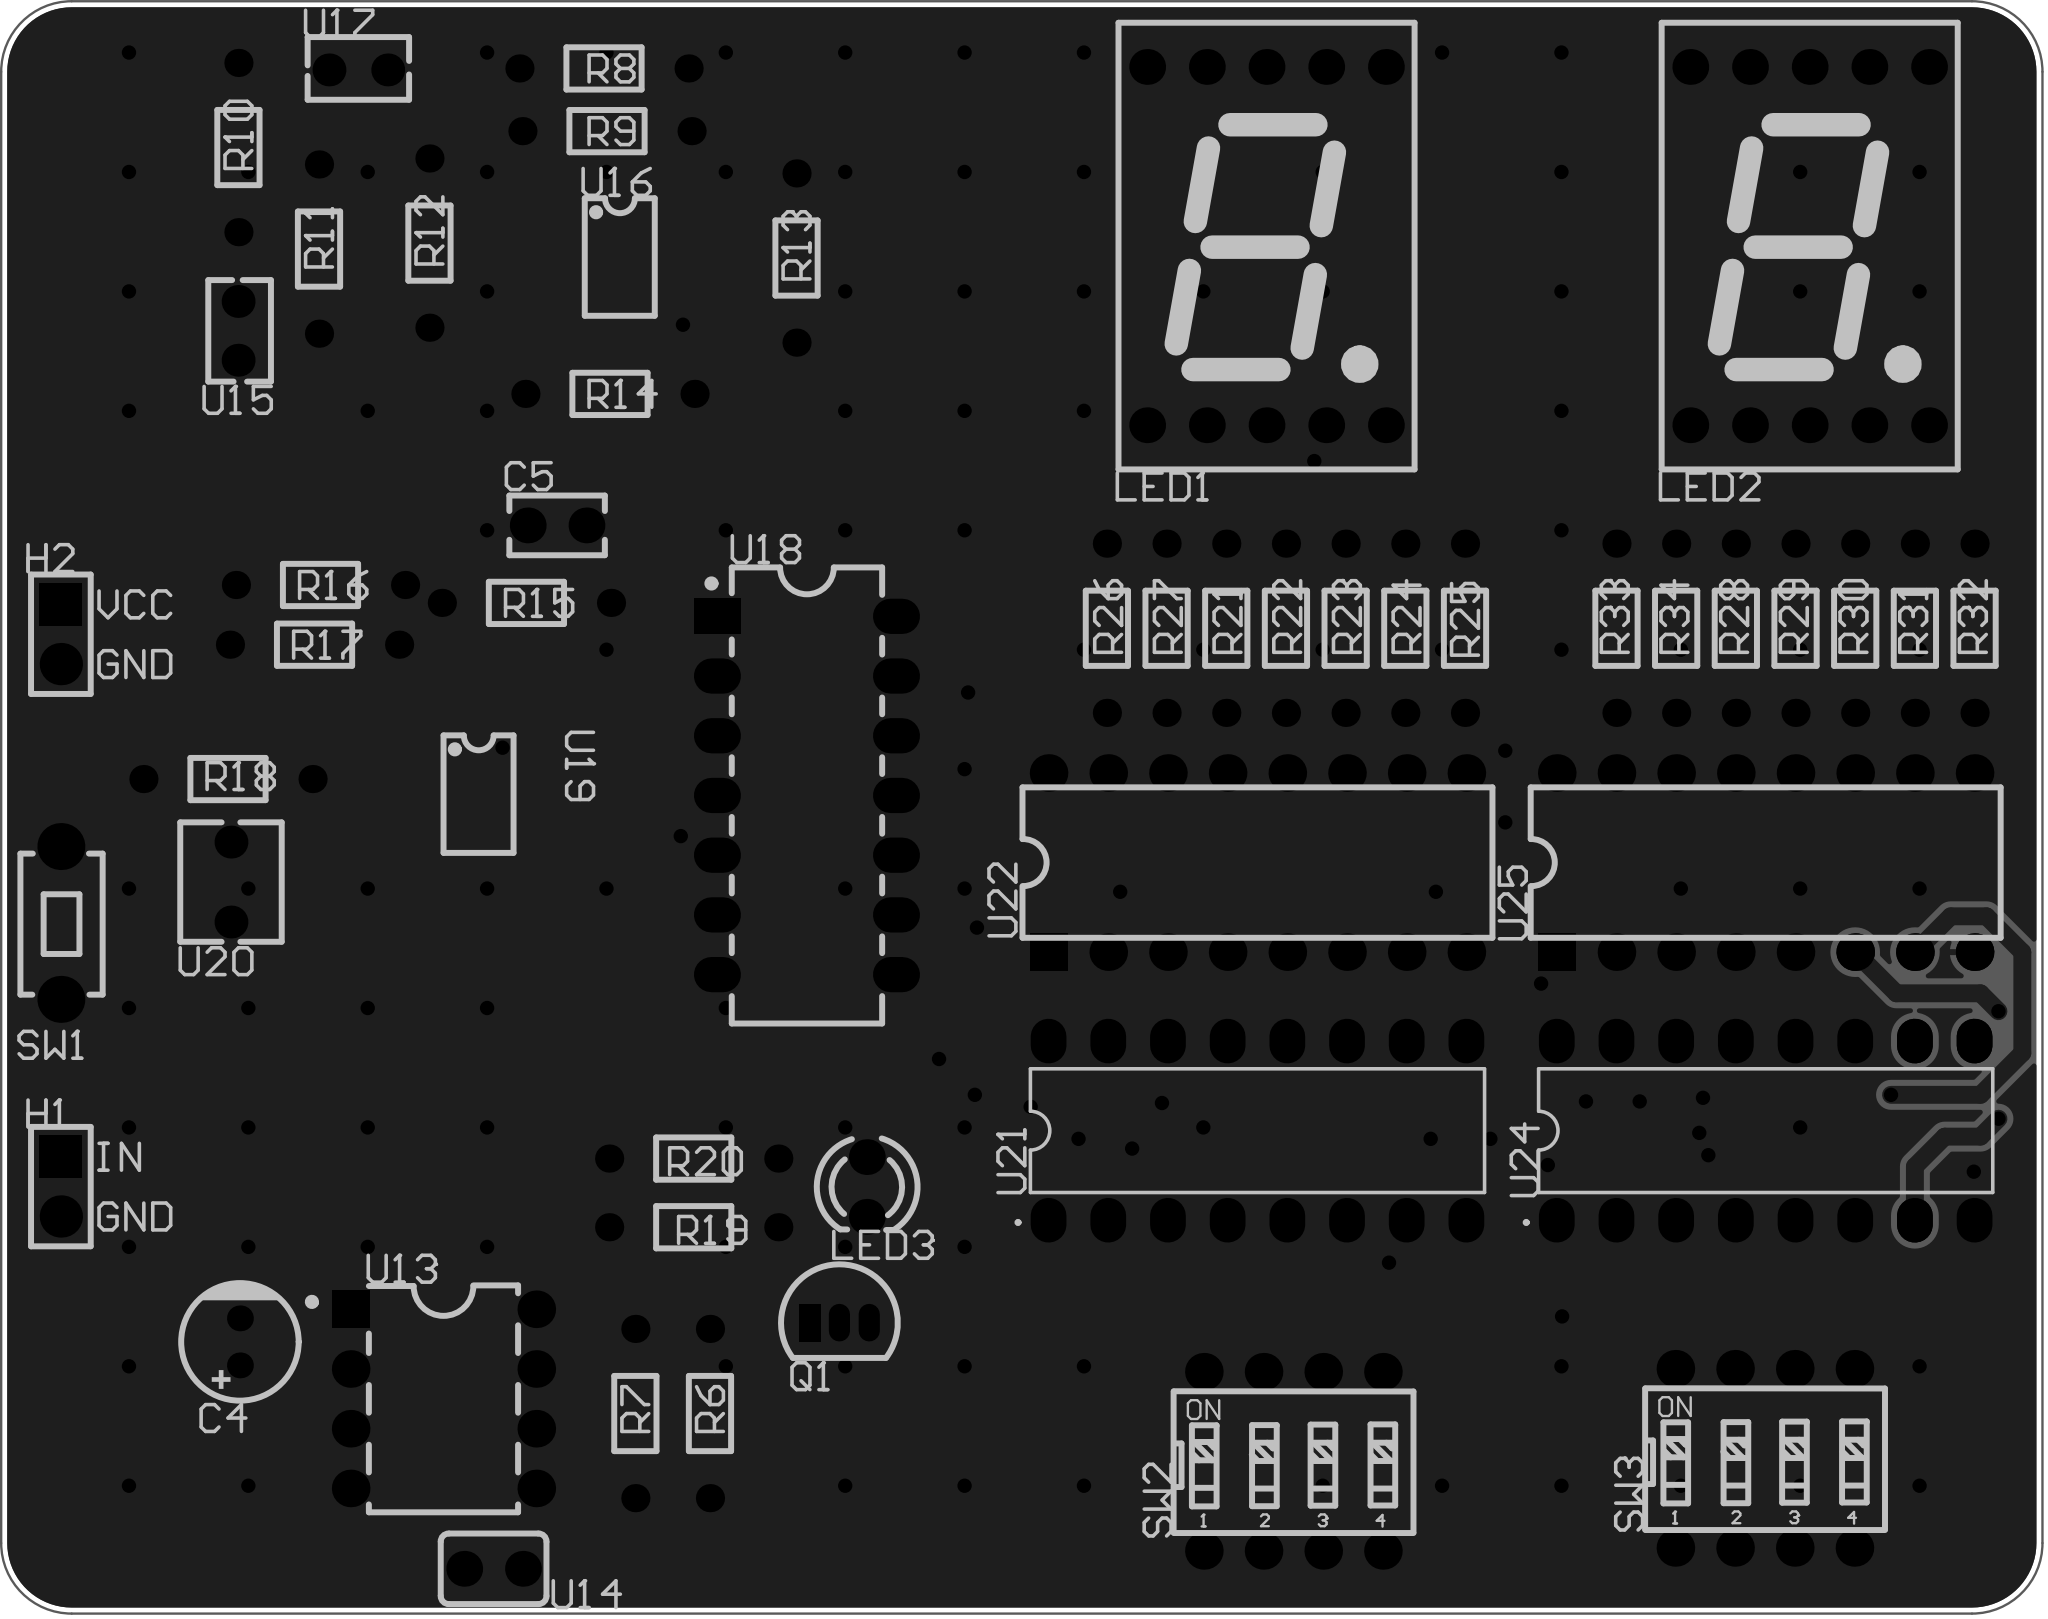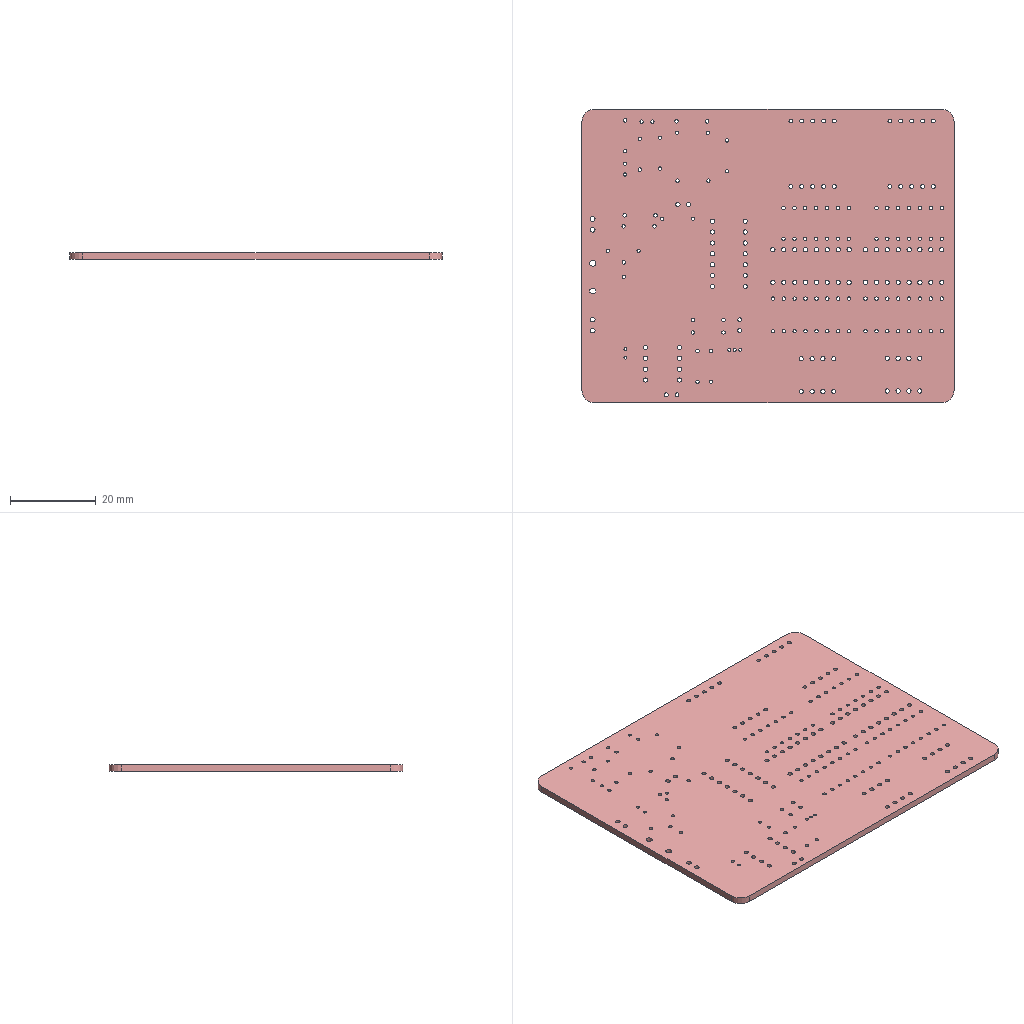Circuit board layout | Altium Designer | box 86.9 x 68.6 x 1.6 mm
Layer stack:
# Altium Designer layer stack of  (unit mm; dielectric type: 0 none, 1 core, 2 prepreg, 3 surface material)
index,name,kind,layer,copper_thickness_mm,dielectric_type,dielectric_thickness_mm,dielectric_material,dielectric_constant
0,Top Paste Mask Layer,other,,,,,,
1,Top Silkscreen Layer,other,,,,,,
2,Top Solder Mask Layer,dielectric,,,3,0.01,,3.3
3,Top Layer,copper,Top Layer,0.035,,,,
4,Dielectric1,dielectric,,,3,1.51,FR4,4.5
5,Bottom Layer,copper,Bottom Layer,0.035,,,,
6,Bottom Solder Mask Layer,dielectric,,,3,0.01,,3.3
7,Bottom Silkscreen Layer,other,,,,,,
8,Bottom Paste Mask Layer,other,,,,,,
# drill layer pairs: low layer,high layer
drill_pair,Top Layer,Bottom Layer
Part placement:
Designator,Comment,Layer,Footprint,Center-X(mm),Center-Y(mm),Rotation
C4,10uF,TopLayer,CAP-TH_BD5.0-P2.00-D0.5-FD,96.774,94.107,90
C5,100nF,TopLayer,CAP-TH_L4.0-W2.5-P2.50-D0.5-A,110.272,128.835,0
H1,,TopLayer,HDR-TH_2P-P2.54-V-M-1,89.154,100.711,270
LED1,,TopLayer,LED-SEG-TH_10P-L12.6-W19.0-P2.54-S15.24-BL,140.462,140.716,0
LED2,,TopLayer,LED-SEG-TH_10P-L12.6-W19.0-P2.54-S15.24-BL,163.576,140.716,0
LED3,,TopLayer,LED_TH-3mm,123.452,100.697,270
Q1,2N2222A,TopLayer,TO-92-3_L4.9-W3.7-P1.27-L,122.285,94.924,0
R6,47kΩ,TopLayer,Res_1/8W,116.777,91.059,90
R7,47kΩ,TopLayer,Res_1/8W,113.602,91.059,90
R8,4.7kΩ,TopLayer,Res_1/8W,112.268,148.272,0
R9,4.7kΩ,TopLayer,Res_1/8W,112.395,145.605,0
R10,4.7kΩ,TopLayer,Res_1/8W,96.71,144.907,270
R11,1kΩ,TopLayer,Res_1/8W,100.139,140.589,270
R12,100kΩ,TopLayer,Res_1/8W,104.839,140.843,90
R13,10kΩ,TopLayer,Res_1/8W,120.46,140.208,90
R14,2kΩ,TopLayer,Res_1/8W,112.522,134.429,0
R15,10kΩ,TopLayer,Res_1/8W,108.966,125.539,0
R16,100kΩ,TopLayer,Res_1/8W,100.203,126.301,0
R17,100kΩ,TopLayer,Res_1/8W,99.949,123.761,0
R18,100kΩ,TopLayer,Res_1/8W,96.266,118.046,0
R19,3kΩ,TopLayer,Res_1/8W,116.086,98.983,180
R20,200Ω,TopLayer,Res_1/8W,116.086,101.904,180
SW1,,TopLayer,Key_TH_3.5x6x4.3,89.154,111.925,90
SW2,拨码开关EI-04,TopLayer,SW-TH_DIPSWITCHEI-04,141.605,89.027,0
SW3,拨码开关EI-04,TopLayer,SW-TH_DIPSWITCHEI-04,161.671,89.154,0
U13,NE555PE4,TopLayer,PDIP-8_L9.6-W6.4-P2.54-LS7.9-BL-1,105.436,91.683,270
U14,100nF,TopLayer,CAP-TH_L4.5-W3.0-P2.50-D0.5,107.569,84.455,0
U15,1uF,TopLayer,CAP-TH_L4.0-W2.5-P2.50-D0.5,96.697,137.11,90
U16,LM358AD,TopLayer,SOP-8_L4.9-W3.9-P1.27-LS6.0-BL,112.946,140.251,270
U17,1uF,TopLayer,CAP-TH_L4.0-W2.5-P2.50-D0.5,101.814,148.209,180
U18,CD4011BD,TopLayer,PDIP-14_L19.3-W6.4-P2.54-LS7.9-BL-1,120.904,117.348,270
U19,LM358AD,TopLayer,SOP-8_L4.9-W3.9-P1.27-LS6.0-BL,106.936,117.405,270
U20,光敏电阻-5MM,TopLayer,RES-TH_L4.9-W4.3-P3.4,96.393,113.665,90
U21,SN74LS190N,TopLayer,PDIP-16_L19.2-W6.6-P2.54-LS7.6-BL,140.076,103.091,0
U22,CD4511BE,TopLayer,DIP-16_L19.8-W6.5-P2.54-LS7.6-BL,140.076,114.494,0
U24,SN74LS190N,TopLayer,PDIP-16_L19.2-W6.6-P2.54-LS7.6-BL,161.703,103.091,0
U25,CD4511BE,TopLayer,DIP-16_L19.8-W6.5-P2.54-LS7.6-BL,161.703,114.494,0
R21,10kΩ,TopLayer,Res_1/8W,138.748,124.46,90
R22,10kΩ,TopLayer,Res_1/8W,141.288,124.46,90
R23,10kΩ,TopLayer,Res_1/8W,143.828,124.46,90
R24,10kΩ,TopLayer,Res_1/8W,146.368,124.46,90
R25,10kΩ,TopLayer,Res_1/8W,148.908,124.46,90
R26,10kΩ,TopLayer,Res_1/8W,133.668,124.46,90
R27,10kΩ,TopLayer,Res_1/8W,136.208,124.46,90
R28,10kΩ,TopLayer,Res_1/8W,160.433,124.46,90
R29,10kΩ,TopLayer,Res_1/8W,162.973,124.46,90
R30,10kΩ,TopLayer,Res_1/8W,165.513,124.46,90
R31,10kΩ,TopLayer,Res_1/8W,168.053,124.46,90
R32,10kΩ,TopLayer,Res_1/8W,170.593,124.46,90
R33,10kΩ,TopLayer,Res_1/8W,155.353,124.46,90
R34,10kΩ,TopLayer,Res_1/8W,157.893,124.46,90
H2,,TopLayer,HDR-TH_2P-P2.54-V-M-1,89.154,124.206,270
Pad and via stacks:
# Altium Designer via and pad stacks of  (unit mm). Each distinct definition once, with the count of objects using it.
# via: kind,start_layer,end_layer,hole_mm,diameter_mm,mode(0 simple;1 top-mid-bottom;2 full stack),diameter_per_layer,count,example_net
# pad: kind,layer,hole_mm,hole_type(0 round;1 square;2 slot),plating,top_size,top_shape(1 round;2 rect;3 octagon;9 rounded rect),mid_size,bottom_size,mode,footprint,size_per_layer,count,example
pad,Multi-Layer,0.7,0,plated,1.1x1.1,1,1.1x1.1,1.1x1.1,0,CAP-TH_BD5.0-P2.00-D0.5-FD,,2,C4.1
pad,Multi-Layer,1,0,plated,1.524x1.524,1,1.524x1.524,1.524x1.524,0,CAP-TH_L4.0-W2.5-P2.50-D0.5-A,,2,C5.1
pad,Multi-Layer,1.1,0,plated,1.8x1.8,1,1.8x1.8,1.8x1.8,0,HDR-TH_2P-P2.54-V-M-1,,2,H1.2
pad,Multi-Layer,1.1,0,plated,1.8x1.8,2,1.8x1.8,1.8x1.8,0,HDR-TH_2P-P2.54-V-M-1,,2,H1.1
pad,Multi-Layer,0.9144,0,plated,1.524x1.524,1,1.524x1.524,1.524x1.524,0,LED-SEG-TH_10P-L12.6-W19.0-P2.54-S15.24-BL,,20,LED1.1
pad,Multi-Layer,0.9144,0,plated,1.524x1.524,1,1.524x1.524,1.524x1.524,0,LED_TH-3mm,,2,LED3.1
pad,Multi-Layer,0.7,0,plated,0.9x1.6,1,0.9x1.6,0.9x1.6,0,TO-92-3_L4.9-W3.7-P1.27-L,,2,Q1.3
pad,Multi-Layer,0.7,0,plated,0.9x1.6,2,0.9x1.6,0.9x1.6,0,TO-92-3_L4.9-W3.7-P1.27-L,,1,Q1.1
pad,Multi-Layer,0.8001,0,plated,1.199x1.199,1,1.199x1.199,1.199x1.199,0,Res_1/8W,,58,R6.1
pad,Multi-Layer,1.399,0,plated,1.999x1.999,1,1.999x1.999,1.999x1.999,0,Key_TH_3.5x6x4.3,,2,SW1.A
pad,Multi-Layer,1,0,plated,1.6x1.6,1,1.6x1.6,1.6x1.6,0,SW-TH_DIPSWITCHEI-04,,16,SW2.1
pad,Multi-Layer,1,0,plated,1.6x1.6,1,1.6x1.6,1.6x1.6,0,PDIP-8_L9.6-W6.4-P2.54-LS7.9-BL-1,,7,U13.8
pad,Multi-Layer,1,0,plated,1.6x1.6,2,1.6x1.6,1.6x1.6,0,PDIP-8_L9.6-W6.4-P2.54-LS7.9-BL-1,,1,U13.1
pad,Multi-Layer,0.9144,0,plated,1.524x1.524,1,1.524x1.524,1.524x1.524,0,CAP-TH_L4.5-W3.0-P2.50-D0.5,,2,U14.1
pad,Multi-Layer,0.8,0,plated,1.4x1.4,1,1.4x1.4,1.4x1.4,0,CAP-TH_L4.0-W2.5-P2.50-D0.5,,4,U15.2
pad,Multi-Layer,1,0,plated,2x1.5,2,2x1.5,2x1.5,0,PDIP-14_L19.3-W6.4-P2.54-LS7.9-BL-1,,1,U18.1
pad,Multi-Layer,1,0,plated,2x1.5,1,2x1.5,2x1.5,0,PDIP-14_L19.3-W6.4-P2.54-LS7.9-BL-1,,13,U18.2
pad,Multi-Layer,0.8,0,plated,1.4x1.4,1,1.4x1.4,1.4x1.4,0,RES-TH_L4.9-W4.3-P3.4,,2,U20.1
pad,Multi-Layer,0.8,0,plated,1.52x1.9,1,1.52x1.9,1.52x1.9,0,PDIP-16_L19.2-W6.6-P2.54-LS7.6-BL,,32,U21.1
pad,Multi-Layer,1,0,plated,1.6x1.6,1,1.6x1.6,1.6x1.6,0,DIP-16_L19.8-W6.5-P2.54-LS7.6-BL,,30,U22.16
pad,Multi-Layer,1,0,plated,1.6x1.6,2,1.6x1.6,1.6x1.6,0,DIP-16_L19.8-W6.5-P2.54-LS7.6-BL,,2,U22.1
pad,Top Layer,0,0,plated,0.63x1.865,1,0.63x1.865,0.63x1.865,0,SOP-8_L4.9-W3.9-P1.27-LS6.0-BL,,16,U16.1
via,Top Layer,Bottom Layer,0.3048,0.61,0,,134,$1N10205
via,Top Layer,Bottom Layer,0.3048,0.6096,0,,1,$1N11115
Copper pours:
name,layer,net,type(0 solid;1 hatched;2 none)
Bottom Layer-GND,Bottom Layer,GND,0
Top Layer-GND,Top Layer,GND,0
Design rules, without the lines most boards share:
# Altium Designer design rules of  (exported by Altium Designer, unit mm)
# columns: name | kind | enabled | priority | scope1 | scope2 | descriptor | typed fields (field=value)
copperThickness1oz_2 | 2 | enabled | 2 | All | All | Width Constraint (Min=5mil) (Max=100mil) (Preferred=30mil) (All) |
viaSize | 11 | enabled | 1 | All | All | Routing Via (MinHoleWidth=11.811mil) (MaxHoleWidth=248.032mil) (PreferredHoleWidth=12.008mil) (MinWidth=19.685mil) (MaxWidth=393.701mil) (PreferedWidth=24.016mil) (All) | via_min_hole=0.3 via_max_hole=6.3 via_preferred_diameter=0.61 via_preferred_hole=0.305
solderMaskExpansion | 13 | enabled | 2 | All | All | Solder Mask Expansion (Expansion =2.008mil) (All) | expansion=0.051